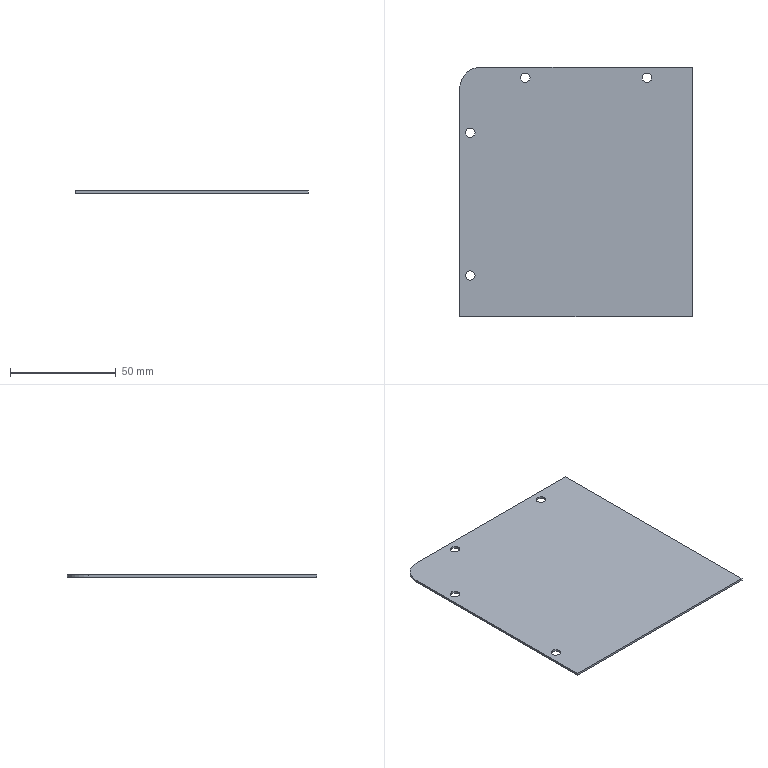Part | SolidWorks | features Cut 1, FlatPattern 1, SMBaseFlange 1, SheetMetal 1 | 1 solid | 15 faces | box 110 x 118 x 1 mm | volume 12895 mm3 | cylinder 9 | plane 6 | commonest cylinder face diameters 4.5 x8 20 x1
STEP:
#1=CARTESIAN_POINT('',(-34.867,-67.507,-1.));
#2=VERTEX_POINT('',#1);
#3=CARTESIAN_POINT('',(-30.367,-67.507,-1.));
#4=VERTEX_POINT('',#3);
#5=CARTESIAN_POINT('',(-32.617,-67.507,-1.));
#6=DIRECTION('',(0.,0.,1.));
#7=DIRECTION('',(1.,0.,0.));
#8=AXIS2_PLACEMENT_3D('',#5,#6,#7);
#9=CIRCLE('',#8,2.25);
#10=EDGE_CURVE('',#2,#4,#9,.T.);
#11=ORIENTED_EDGE('',*,*,#10,.F.);
#12=CARTESIAN_POINT('',(-34.867,-67.507,0.));
#13=VERTEX_POINT('',#12);
#14=CARTESIAN_POINT('',(-34.867,-67.507,-1.));
#15=DIRECTION('',(0.,0.,1.));
#16=VECTOR('',#15,1000.);
#17=LINE('',#14,#16);
#18=EDGE_CURVE('',#2,#13,#17,.T.);
#19=ORIENTED_EDGE('',*,*,#18,.T.);
#20=CARTESIAN_POINT('',(-30.367,-67.507,0.));
#21=VERTEX_POINT('',#20);
#22=CARTESIAN_POINT('',(-32.617,-67.507,0.));
#23=DIRECTION('',(0.,0.,1.));
#24=DIRECTION('',(1.,0.,0.));
#25=AXIS2_PLACEMENT_3D('',#22,#23,#24);
#26=CIRCLE('',#25,2.25);
#27=EDGE_CURVE('',#13,#21,#26,.T.);
#28=ORIENTED_EDGE('',*,*,#27,.T.);
#29=CARTESIAN_POINT('',(-30.367,-67.507,-1.));
#30=DIRECTION('',(0.,0.,1.));
#31=VECTOR('',#30,1000.);
#32=LINE('',#29,#31);
#33=EDGE_CURVE('',#4,#21,#32,.T.);
#34=ORIENTED_EDGE('',*,*,#33,.F.);
#35=EDGE_LOOP('',(#11,#19,#28,#34));
#36=FACE_OUTER_BOUND('',#35,.T.);
#37=CARTESIAN_POINT('',(-32.617,-67.507,-1.));
#38=DIRECTION('',(0.,0.,1.));
#39=DIRECTION('',(1.,0.,0.));
#40=AXIS2_PLACEMENT_3D('',#37,#38,#39);
#41=CYLINDRICAL_SURFACE('',#40,2.25);
#42=ADVANCED_FACE('',(#36),#41,.F.);
#43=CARTESIAN_POINT('',(-34.867,-0.007086,-1.));
#44=VERTEX_POINT('',#43);
#45=CARTESIAN_POINT('',(-30.367,-0.007086,-1.));
#46=VERTEX_POINT('',#45);
#47=CARTESIAN_POINT('',(-32.617,-0.007086,-1.));
#48=DIRECTION('',(0.,0.,1.));
#49=DIRECTION('',(1.,0.,0.));
#50=AXIS2_PLACEMENT_3D('',#47,#48,#49);
#51=CIRCLE('',#50,2.25);
#52=EDGE_CURVE('',#44,#46,#51,.T.);
#53=ORIENTED_EDGE('',*,*,#52,.F.);
#54=CARTESIAN_POINT('',(-34.867,-0.007086,0.));
#55=VERTEX_POINT('',#54);
#56=CARTESIAN_POINT('',(-34.867,-0.007086,-1.));
#57=DIRECTION('',(0.,0.,1.));
#58=VECTOR('',#57,1000.);
#59=LINE('',#56,#58);
#60=EDGE_CURVE('',#44,#55,#59,.T.);
#61=ORIENTED_EDGE('',*,*,#60,.T.);
#62=CARTESIAN_POINT('',(-30.367,-0.007086,0.));
#63=VERTEX_POINT('',#62);
#64=CARTESIAN_POINT('',(-32.617,-0.007086,0.));
#65=DIRECTION('',(0.,0.,1.));
#66=DIRECTION('',(1.,0.,0.));
#67=AXIS2_PLACEMENT_3D('',#64,#65,#66);
#68=CIRCLE('',#67,2.25);
#69=EDGE_CURVE('',#55,#63,#68,.T.);
#70=ORIENTED_EDGE('',*,*,#69,.T.);
#71=CARTESIAN_POINT('',(-30.367,-0.007086,-1.));
#72=DIRECTION('',(0.,0.,1.));
#73=VECTOR('',#72,1000.);
#74=LINE('',#71,#73);
#75=EDGE_CURVE('',#46,#63,#74,.T.);
#76=ORIENTED_EDGE('',*,*,#75,.F.);
#77=EDGE_LOOP('',(#53,#61,#70,#76));
#78=FACE_OUTER_BOUND('',#77,.T.);
#79=CARTESIAN_POINT('',(-32.617,-0.007086,-1.));
#80=DIRECTION('',(0.,0.,1.));
#81=DIRECTION('',(1.,0.,0.));
#82=AXIS2_PLACEMENT_3D('',#79,#80,#81);
#83=CYLINDRICAL_SURFACE('',#82,2.25);
#84=ADVANCED_FACE('',(#78),#83,.F.);
#85=CARTESIAN_POINT('',(-8.867,25.993,-1.));
#86=VERTEX_POINT('',#85);
#87=CARTESIAN_POINT('',(-4.367,25.993,-1.));
#88=VERTEX_POINT('',#87);
#89=CARTESIAN_POINT('',(-6.617,25.993,-1.));
#90=DIRECTION('',(0.,0.,1.));
#91=DIRECTION('',(1.,0.,0.));
#92=AXIS2_PLACEMENT_3D('',#89,#90,#91);
#93=CIRCLE('',#92,2.25);
#94=EDGE_CURVE('',#86,#88,#93,.T.);
#95=ORIENTED_EDGE('',*,*,#94,.F.);
#96=CARTESIAN_POINT('',(-8.867,25.993,0.));
#97=VERTEX_POINT('',#96);
#98=CARTESIAN_POINT('',(-8.867,25.993,-1.));
#99=DIRECTION('',(0.,0.,1.));
#100=VECTOR('',#99,1000.);
#101=LINE('',#98,#100);
#102=EDGE_CURVE('',#86,#97,#101,.T.);
#103=ORIENTED_EDGE('',*,*,#102,.T.);
#104=CARTESIAN_POINT('',(-4.367,25.993,0.));
#105=VERTEX_POINT('',#104);
#106=CARTESIAN_POINT('',(-6.617,25.993,0.));
#107=DIRECTION('',(0.,0.,1.));
#108=DIRECTION('',(1.,0.,0.));
#109=AXIS2_PLACEMENT_3D('',#106,#107,#108);
#110=CIRCLE('',#109,2.25);
#111=EDGE_CURVE('',#97,#105,#110,.T.);
#112=ORIENTED_EDGE('',*,*,#111,.T.);
#113=CARTESIAN_POINT('',(-4.367,25.993,-1.));
#114=DIRECTION('',(0.,0.,1.));
#115=VECTOR('',#114,1000.);
#116=LINE('',#113,#115);
#117=EDGE_CURVE('',#88,#105,#116,.T.);
#118=ORIENTED_EDGE('',*,*,#117,.F.);
#119=EDGE_LOOP('',(#95,#103,#112,#118));
#120=FACE_OUTER_BOUND('',#119,.T.);
#121=CARTESIAN_POINT('',(-6.617,25.993,-1.));
#122=DIRECTION('',(0.,0.,1.));
#123=DIRECTION('',(1.,0.,0.));
#124=AXIS2_PLACEMENT_3D('',#121,#122,#123);
#125=CYLINDRICAL_SURFACE('',#124,2.25);
#126=ADVANCED_FACE('',(#120),#125,.F.);
#127=CARTESIAN_POINT('',(48.633,25.993,-1.));
#128=VERTEX_POINT('',#127);
#129=CARTESIAN_POINT('',(53.133,25.993,-1.));
#130=VERTEX_POINT('',#129);
#131=CARTESIAN_POINT('',(50.883,25.993,-1.));
#132=DIRECTION('',(0.,0.,1.));
#133=DIRECTION('',(1.,0.,0.));
#134=AXIS2_PLACEMENT_3D('',#131,#132,#133);
#135=CIRCLE('',#134,2.25);
#136=EDGE_CURVE('',#128,#130,#135,.T.);
#137=ORIENTED_EDGE('',*,*,#136,.F.);
#138=CARTESIAN_POINT('',(48.633,25.993,0.));
#139=VERTEX_POINT('',#138);
#140=CARTESIAN_POINT('',(48.633,25.993,-1.));
#141=DIRECTION('',(0.,0.,1.));
#142=VECTOR('',#141,1000.);
#143=LINE('',#140,#142);
#144=EDGE_CURVE('',#128,#139,#143,.T.);
#145=ORIENTED_EDGE('',*,*,#144,.T.);
#146=CARTESIAN_POINT('',(53.133,25.993,0.));
#147=VERTEX_POINT('',#146);
#148=CARTESIAN_POINT('',(50.883,25.993,0.));
#149=DIRECTION('',(0.,0.,1.));
#150=DIRECTION('',(1.,0.,0.));
#151=AXIS2_PLACEMENT_3D('',#148,#149,#150);
#152=CIRCLE('',#151,2.25);
#153=EDGE_CURVE('',#139,#147,#152,.T.);
#154=ORIENTED_EDGE('',*,*,#153,.T.);
#155=CARTESIAN_POINT('',(53.133,25.993,-1.));
#156=DIRECTION('',(0.,0.,1.));
#157=VECTOR('',#156,1000.);
#158=LINE('',#155,#157);
#159=EDGE_CURVE('',#130,#147,#158,.T.);
#160=ORIENTED_EDGE('',*,*,#159,.F.);
#161=EDGE_LOOP('',(#137,#145,#154,#160));
#162=FACE_OUTER_BOUND('',#161,.T.);
#163=CARTESIAN_POINT('',(50.883,25.993,-1.));
#164=DIRECTION('',(0.,0.,1.));
#165=DIRECTION('',(1.,0.,0.));
#166=AXIS2_PLACEMENT_3D('',#163,#164,#165);
#167=CYLINDRICAL_SURFACE('',#166,2.25);
#168=ADVANCED_FACE('',(#162),#167,.F.);
#169=CARTESIAN_POINT('',(72.383,-87.007,0.));
#170=VERTEX_POINT('',#169);
#171=CARTESIAN_POINT('',(72.383,30.993,0.));
#172=VERTEX_POINT('',#171);
#173=CARTESIAN_POINT('',(72.383,30.993,0.));
#174=DIRECTION('',(0.,1.,0.));
#175=VECTOR('',#174,1000.);
#176=LINE('',#173,#175);
#177=EDGE_CURVE('',#170,#172,#176,.T.);
#178=ORIENTED_EDGE('',*,*,#177,.F.);
#179=CARTESIAN_POINT('',(72.383,-87.007,-1.));
#180=VERTEX_POINT('',#179);
#181=CARTESIAN_POINT('',(72.383,-87.007,-1.));
#182=DIRECTION('',(0.,0.,1.));
#183=VECTOR('',#182,1000.);
#184=LINE('',#181,#183);
#185=EDGE_CURVE('',#180,#170,#184,.T.);
#186=ORIENTED_EDGE('',*,*,#185,.F.);
#187=CARTESIAN_POINT('',(72.383,30.993,-1.));
#188=VERTEX_POINT('',#187);
#189=CARTESIAN_POINT('',(72.383,30.993,-1.));
#190=DIRECTION('',(0.,1.,0.));
#191=VECTOR('',#190,1000.);
#192=LINE('',#189,#191);
#193=EDGE_CURVE('',#180,#188,#192,.T.);
#194=ORIENTED_EDGE('',*,*,#193,.T.);
#195=CARTESIAN_POINT('',(72.383,30.993,-1.));
#196=DIRECTION('',(0.,0.,1.));
#197=VECTOR('',#196,1000.);
#198=LINE('',#195,#197);
#199=EDGE_CURVE('',#188,#172,#198,.T.);
#200=ORIENTED_EDGE('',*,*,#199,.T.);
#201=EDGE_LOOP('',(#178,#186,#194,#200));
#202=FACE_OUTER_BOUND('',#201,.T.);
#203=CARTESIAN_POINT('',(72.383,30.993,-1.));
#204=DIRECTION('',(1.,0.,0.));
#205=DIRECTION('',(0.,1.,0.));
#206=AXIS2_PLACEMENT_3D('',#203,#204,#205);
#207=PLANE('',#206);
#208=ADVANCED_FACE('',(#202),#207,.T.);
#209=CARTESIAN_POINT('',(-37.617,-87.007,0.));
#210=VERTEX_POINT('',#209);
#211=CARTESIAN_POINT('',(-37.617,-87.007,0.));
#212=DIRECTION('',(1.,0.,0.));
#213=VECTOR('',#212,1000.);
#214=LINE('',#211,#213);
#215=EDGE_CURVE('',#210,#170,#214,.T.);
#216=ORIENTED_EDGE('',*,*,#215,.F.);
#217=CARTESIAN_POINT('',(-37.617,-87.007,-1.));
#218=VERTEX_POINT('',#217);
#219=CARTESIAN_POINT('',(-37.617,-87.007,-1.));
#220=DIRECTION('',(0.,0.,1.));
#221=VECTOR('',#220,1000.);
#222=LINE('',#219,#221);
#223=EDGE_CURVE('',#218,#210,#222,.T.);
#224=ORIENTED_EDGE('',*,*,#223,.F.);
#225=CARTESIAN_POINT('',(-37.617,-87.007,-1.));
#226=DIRECTION('',(1.,0.,0.));
#227=VECTOR('',#226,1000.);
#228=LINE('',#225,#227);
#229=EDGE_CURVE('',#218,#180,#228,.T.);
#230=ORIENTED_EDGE('',*,*,#229,.T.);
#231=ORIENTED_EDGE('',*,*,#185,.T.);
#232=EDGE_LOOP('',(#216,#224,#230,#231));
#233=FACE_OUTER_BOUND('',#232,.T.);
#234=CARTESIAN_POINT('',(-37.617,-87.007,-1.));
#235=DIRECTION('',(0.,-1.,0.));
#236=DIRECTION('',(0.,0.,-1.));
#237=AXIS2_PLACEMENT_3D('',#234,#235,#236);
#238=PLANE('',#237);
#239=ADVANCED_FACE('',(#233),#238,.T.);
#240=CARTESIAN_POINT('',(-37.617,20.993,0.));
#241=VERTEX_POINT('',#240);
#242=CARTESIAN_POINT('',(-37.617,20.993,0.));
#243=DIRECTION('',(0.,-1.,0.));
#244=VECTOR('',#243,1000.);
#245=LINE('',#242,#244);
#246=EDGE_CURVE('',#241,#210,#245,.T.);
#247=ORIENTED_EDGE('',*,*,#246,.F.);
#248=CARTESIAN_POINT('',(-37.617,20.993,-1.));
#249=VERTEX_POINT('',#248);
#250=CARTESIAN_POINT('',(-37.617,20.993,-1.));
#251=DIRECTION('',(0.,0.,1.));
#252=VECTOR('',#251,1000.);
#253=LINE('',#250,#252);
#254=EDGE_CURVE('',#249,#241,#253,.T.);
#255=ORIENTED_EDGE('',*,*,#254,.F.);
#256=CARTESIAN_POINT('',(-37.617,20.993,-1.));
#257=DIRECTION('',(0.,-1.,0.));
#258=VECTOR('',#257,1000.);
#259=LINE('',#256,#258);
#260=EDGE_CURVE('',#249,#218,#259,.T.);
#261=ORIENTED_EDGE('',*,*,#260,.T.);
#262=ORIENTED_EDGE('',*,*,#223,.T.);
#263=EDGE_LOOP('',(#247,#255,#261,#262));
#264=FACE_OUTER_BOUND('',#263,.T.);
#265=CARTESIAN_POINT('',(-37.617,20.993,-1.));
#266=DIRECTION('',(-1.,0.,0.));
#267=DIRECTION('',(0.,-1.,0.));
#268=AXIS2_PLACEMENT_3D('',#265,#266,#267);
#269=PLANE('',#268);
#270=ADVANCED_FACE('',(#264),#269,.T.);
#271=CARTESIAN_POINT('',(-27.617,30.993,0.));
#272=VERTEX_POINT('',#271);
#273=CARTESIAN_POINT('',(-27.617,20.993,0.));
#274=DIRECTION('',(0.,0.,1.));
#275=DIRECTION('',(1.,0.,0.));
#276=AXIS2_PLACEMENT_3D('',#273,#274,#275);
#277=CIRCLE('',#276,10.);
#278=EDGE_CURVE('',#272,#241,#277,.T.);
#279=ORIENTED_EDGE('',*,*,#278,.F.);
#280=CARTESIAN_POINT('',(-27.617,30.993,-1.));
#281=VERTEX_POINT('',#280);
#282=CARTESIAN_POINT('',(-27.617,30.993,-1.));
#283=DIRECTION('',(0.,0.,1.));
#284=VECTOR('',#283,1000.);
#285=LINE('',#282,#284);
#286=EDGE_CURVE('',#281,#272,#285,.T.);
#287=ORIENTED_EDGE('',*,*,#286,.F.);
#288=CARTESIAN_POINT('',(-27.617,20.993,-1.));
#289=DIRECTION('',(0.,0.,1.));
#290=DIRECTION('',(1.,0.,0.));
#291=AXIS2_PLACEMENT_3D('',#288,#289,#290);
#292=CIRCLE('',#291,10.);
#293=EDGE_CURVE('',#281,#249,#292,.T.);
#294=ORIENTED_EDGE('',*,*,#293,.T.);
#295=ORIENTED_EDGE('',*,*,#254,.T.);
#296=EDGE_LOOP('',(#279,#287,#294,#295));
#297=FACE_OUTER_BOUND('',#296,.T.);
#298=CARTESIAN_POINT('',(-27.617,20.993,-1.));
#299=DIRECTION('',(0.,0.,1.));
#300=DIRECTION('',(1.,0.,0.));
#301=AXIS2_PLACEMENT_3D('',#298,#299,#300);
#302=CYLINDRICAL_SURFACE('',#301,10.);
#303=ADVANCED_FACE('',(#297),#302,.T.);
#304=CARTESIAN_POINT('',(-27.617,30.993,0.));
#305=DIRECTION('',(-1.,0.,0.));
#306=VECTOR('',#305,1000.);
#307=LINE('',#304,#306);
#308=EDGE_CURVE('',#172,#272,#307,.T.);
#309=ORIENTED_EDGE('',*,*,#308,.F.);
#310=ORIENTED_EDGE('',*,*,#199,.F.);
#311=CARTESIAN_POINT('',(-27.617,30.993,-1.));
#312=DIRECTION('',(-1.,0.,0.));
#313=VECTOR('',#312,1000.);
#314=LINE('',#311,#313);
#315=EDGE_CURVE('',#188,#281,#314,.T.);
#316=ORIENTED_EDGE('',*,*,#315,.T.);
#317=ORIENTED_EDGE('',*,*,#286,.T.);
#318=EDGE_LOOP('',(#309,#310,#316,#317));
#319=FACE_OUTER_BOUND('',#318,.T.);
#320=CARTESIAN_POINT('',(-27.617,30.993,-1.));
#321=DIRECTION('',(0.,1.,0.));
#322=DIRECTION('',(0.,0.,1.));
#323=AXIS2_PLACEMENT_3D('',#320,#321,#322);
#324=PLANE('',#323);
#325=ADVANCED_FACE('',(#319),#324,.T.);
#326=CARTESIAN_POINT('',(-32.617,-67.507,-1.));
#327=DIRECTION('',(0.,0.,1.));
#328=DIRECTION('',(1.,0.,0.));
#329=AXIS2_PLACEMENT_3D('',#326,#327,#328);
#330=CIRCLE('',#329,2.25);
#331=EDGE_CURVE('',#4,#2,#330,.T.);
#332=ORIENTED_EDGE('',*,*,#331,.T.);
#333=ORIENTED_EDGE('',*,*,#10,.T.);
#334=EDGE_LOOP('',(#332,#333));
#335=FACE_BOUND('',#334,.T.);
#336=CARTESIAN_POINT('',(-32.617,-0.007086,-1.));
#337=DIRECTION('',(0.,0.,1.));
#338=DIRECTION('',(1.,0.,0.));
#339=AXIS2_PLACEMENT_3D('',#336,#337,#338);
#340=CIRCLE('',#339,2.25);
#341=EDGE_CURVE('',#46,#44,#340,.T.);
#342=ORIENTED_EDGE('',*,*,#341,.T.);
#343=ORIENTED_EDGE('',*,*,#52,.T.);
#344=EDGE_LOOP('',(#342,#343));
#345=FACE_BOUND('',#344,.T.);
#346=CARTESIAN_POINT('',(-6.617,25.993,-1.));
#347=DIRECTION('',(0.,0.,1.));
#348=DIRECTION('',(1.,0.,0.));
#349=AXIS2_PLACEMENT_3D('',#346,#347,#348);
#350=CIRCLE('',#349,2.25);
#351=EDGE_CURVE('',#88,#86,#350,.T.);
#352=ORIENTED_EDGE('',*,*,#351,.T.);
#353=ORIENTED_EDGE('',*,*,#94,.T.);
#354=EDGE_LOOP('',(#352,#353));
#355=FACE_BOUND('',#354,.T.);
#356=CARTESIAN_POINT('',(50.883,25.993,-1.));
#357=DIRECTION('',(0.,0.,1.));
#358=DIRECTION('',(1.,0.,0.));
#359=AXIS2_PLACEMENT_3D('',#356,#357,#358);
#360=CIRCLE('',#359,2.25);
#361=EDGE_CURVE('',#130,#128,#360,.T.);
#362=ORIENTED_EDGE('',*,*,#361,.T.);
#363=ORIENTED_EDGE('',*,*,#136,.T.);
#364=EDGE_LOOP('',(#362,#363));
#365=FACE_BOUND('',#364,.T.);
#366=ORIENTED_EDGE('',*,*,#193,.F.);
#367=ORIENTED_EDGE('',*,*,#229,.F.);
#368=ORIENTED_EDGE('',*,*,#260,.F.);
#369=ORIENTED_EDGE('',*,*,#293,.F.);
#370=ORIENTED_EDGE('',*,*,#315,.F.);
#371=EDGE_LOOP('',(#366,#367,#368,#369,#370));
#372=FACE_OUTER_BOUND('',#371,.T.);
#373=CARTESIAN_POINT('',(-27.617,20.993,-1.));
#374=DIRECTION('',(0.,0.,1.));
#375=DIRECTION('',(1.,0.,0.));
#376=AXIS2_PLACEMENT_3D('',#373,#374,#375);
#377=PLANE('',#376);
#378=ADVANCED_FACE('',(#335,#345,#355,#365,#372),#377,.F.);
#379=CARTESIAN_POINT('',(-32.617,-67.507,0.));
#380=DIRECTION('',(0.,0.,1.));
#381=DIRECTION('',(1.,0.,0.));
#382=AXIS2_PLACEMENT_3D('',#379,#380,#381);
#383=CIRCLE('',#382,2.25);
#384=EDGE_CURVE('',#21,#13,#383,.T.);
#385=ORIENTED_EDGE('',*,*,#384,.F.);
#386=ORIENTED_EDGE('',*,*,#27,.F.);
#387=EDGE_LOOP('',(#385,#386));
#388=FACE_BOUND('',#387,.T.);
#389=CARTESIAN_POINT('',(-32.617,-0.007086,0.));
#390=DIRECTION('',(0.,0.,1.));
#391=DIRECTION('',(1.,0.,0.));
#392=AXIS2_PLACEMENT_3D('',#389,#390,#391);
#393=CIRCLE('',#392,2.25);
#394=EDGE_CURVE('',#63,#55,#393,.T.);
#395=ORIENTED_EDGE('',*,*,#394,.F.);
#396=ORIENTED_EDGE('',*,*,#69,.F.);
#397=EDGE_LOOP('',(#395,#396));
#398=FACE_BOUND('',#397,.T.);
#399=CARTESIAN_POINT('',(-6.617,25.993,0.));
#400=DIRECTION('',(0.,0.,1.));
#401=DIRECTION('',(1.,0.,0.));
#402=AXIS2_PLACEMENT_3D('',#399,#400,#401);
#403=CIRCLE('',#402,2.25);
#404=EDGE_CURVE('',#105,#97,#403,.T.);
#405=ORIENTED_EDGE('',*,*,#404,.F.);
#406=ORIENTED_EDGE('',*,*,#111,.F.);
#407=EDGE_LOOP('',(#405,#406));
#408=FACE_BOUND('',#407,.T.);
#409=CARTESIAN_POINT('',(50.883,25.993,0.));
#410=DIRECTION('',(0.,0.,1.));
#411=DIRECTION('',(1.,0.,0.));
#412=AXIS2_PLACEMENT_3D('',#409,#410,#411);
#413=CIRCLE('',#412,2.25);
#414=EDGE_CURVE('',#147,#139,#413,.T.);
#415=ORIENTED_EDGE('',*,*,#414,.F.);
#416=ORIENTED_EDGE('',*,*,#153,.F.);
#417=EDGE_LOOP('',(#415,#416));
#418=FACE_BOUND('',#417,.T.);
#419=ORIENTED_EDGE('',*,*,#177,.T.);
#420=ORIENTED_EDGE('',*,*,#308,.T.);
#421=ORIENTED_EDGE('',*,*,#278,.T.);
#422=ORIENTED_EDGE('',*,*,#246,.T.);
#423=ORIENTED_EDGE('',*,*,#215,.T.);
#424=EDGE_LOOP('',(#419,#420,#421,#422,#423));
#425=FACE_OUTER_BOUND('',#424,.T.);
#426=CARTESIAN_POINT('',(-27.617,20.993,0.));
#427=DIRECTION('',(0.,0.,1.));
#428=DIRECTION('',(1.,0.,0.));
#429=AXIS2_PLACEMENT_3D('',#426,#427,#428);
#430=PLANE('',#429);
#431=ADVANCED_FACE('',(#388,#398,#408,#418,#425),#430,.T.);
#432=ORIENTED_EDGE('',*,*,#144,.F.);
#433=ORIENTED_EDGE('',*,*,#361,.F.);
#434=ORIENTED_EDGE('',*,*,#159,.T.);
#435=ORIENTED_EDGE('',*,*,#414,.T.);
#436=EDGE_LOOP('',(#432,#433,#434,#435));
#437=FACE_OUTER_BOUND('',#436,.T.);
#438=CARTESIAN_POINT('',(50.883,25.993,-1.));
#439=DIRECTION('',(0.,0.,1.));
#440=DIRECTION('',(1.,0.,0.));
#441=AXIS2_PLACEMENT_3D('',#438,#439,#440);
#442=CYLINDRICAL_SURFACE('',#441,2.25);
#443=ADVANCED_FACE('',(#437),#442,.F.);
#444=ORIENTED_EDGE('',*,*,#102,.F.);
#445=ORIENTED_EDGE('',*,*,#351,.F.);
#446=ORIENTED_EDGE('',*,*,#117,.T.);
#447=ORIENTED_EDGE('',*,*,#404,.T.);
#448=EDGE_LOOP('',(#444,#445,#446,#447));
#449=FACE_OUTER_BOUND('',#448,.T.);
#450=CARTESIAN_POINT('',(-6.617,25.993,-1.));
#451=DIRECTION('',(0.,0.,1.));
#452=DIRECTION('',(1.,0.,0.));
#453=AXIS2_PLACEMENT_3D('',#450,#451,#452);
#454=CYLINDRICAL_SURFACE('',#453,2.25);
#455=ADVANCED_FACE('',(#449),#454,.F.);
#456=ORIENTED_EDGE('',*,*,#60,.F.);
#457=ORIENTED_EDGE('',*,*,#341,.F.);
#458=ORIENTED_EDGE('',*,*,#75,.T.);
#459=ORIENTED_EDGE('',*,*,#394,.T.);
#460=EDGE_LOOP('',(#456,#457,#458,#459));
#461=FACE_OUTER_BOUND('',#460,.T.);
#462=CARTESIAN_POINT('',(-32.617,-0.007086,-1.));
#463=DIRECTION('',(0.,0.,1.));
#464=DIRECTION('',(1.,0.,0.));
#465=AXIS2_PLACEMENT_3D('',#462,#463,#464);
#466=CYLINDRICAL_SURFACE('',#465,2.25);
#467=ADVANCED_FACE('',(#461),#466,.F.);
#468=ORIENTED_EDGE('',*,*,#18,.F.);
#469=ORIENTED_EDGE('',*,*,#331,.F.);
#470=ORIENTED_EDGE('',*,*,#33,.T.);
#471=ORIENTED_EDGE('',*,*,#384,.T.);
#472=EDGE_LOOP('',(#468,#469,#470,#471));
#473=FACE_OUTER_BOUND('',#472,.T.);
#474=CARTESIAN_POINT('',(-32.617,-67.507,-1.));
#475=DIRECTION('',(0.,0.,1.));
#476=DIRECTION('',(1.,0.,0.));
#477=AXIS2_PLACEMENT_3D('',#474,#475,#476);
#478=CYLINDRICAL_SURFACE('',#477,2.25);
#479=ADVANCED_FACE('',(#473),#478,.F.);
#480=CLOSED_SHELL('',(#42,#84,#126,#168,#208,#239,#270,#303,#325,#378,#431,#443,#455,#467,#479));
#481=MANIFOLD_SOLID_BREP('',#480);
#482=CARTESIAN_POINT('',(0.,0.,0.));
#483=DIRECTION('',(0.,0.,1.));
#484=DIRECTION('',(1.,0.,0.));
#485=AXIS2_PLACEMENT_3D('',#482,#483,#484);
#486=(LENGTH_UNIT()NAMED_UNIT(*)SI_UNIT(.MILLI.,.METRE.));
#487=UNCERTAINTY_MEASURE_WITH_UNIT(LENGTH_MEASURE(0.00001),#486,'','');
#488=(NAMED_UNIT(*)PLANE_ANGLE_UNIT()SI_UNIT($,.RADIAN.));
#489=(NAMED_UNIT(*)SI_UNIT($,.STERADIAN.)SOLID_ANGLE_UNIT());
#490=(GEOMETRIC_REPRESENTATION_CONTEXT(3)GLOBAL_UNCERTAINTY_ASSIGNED_CONTEXT((#487))GLOBAL_UNIT_ASSIGNED_CONTEXT((#486,#488,#489))REPRESENTATION_CONTEXT('',''));
#491=ADVANCED_BREP_SHAPE_REPRESENTATION('',(#481,#485),#490);